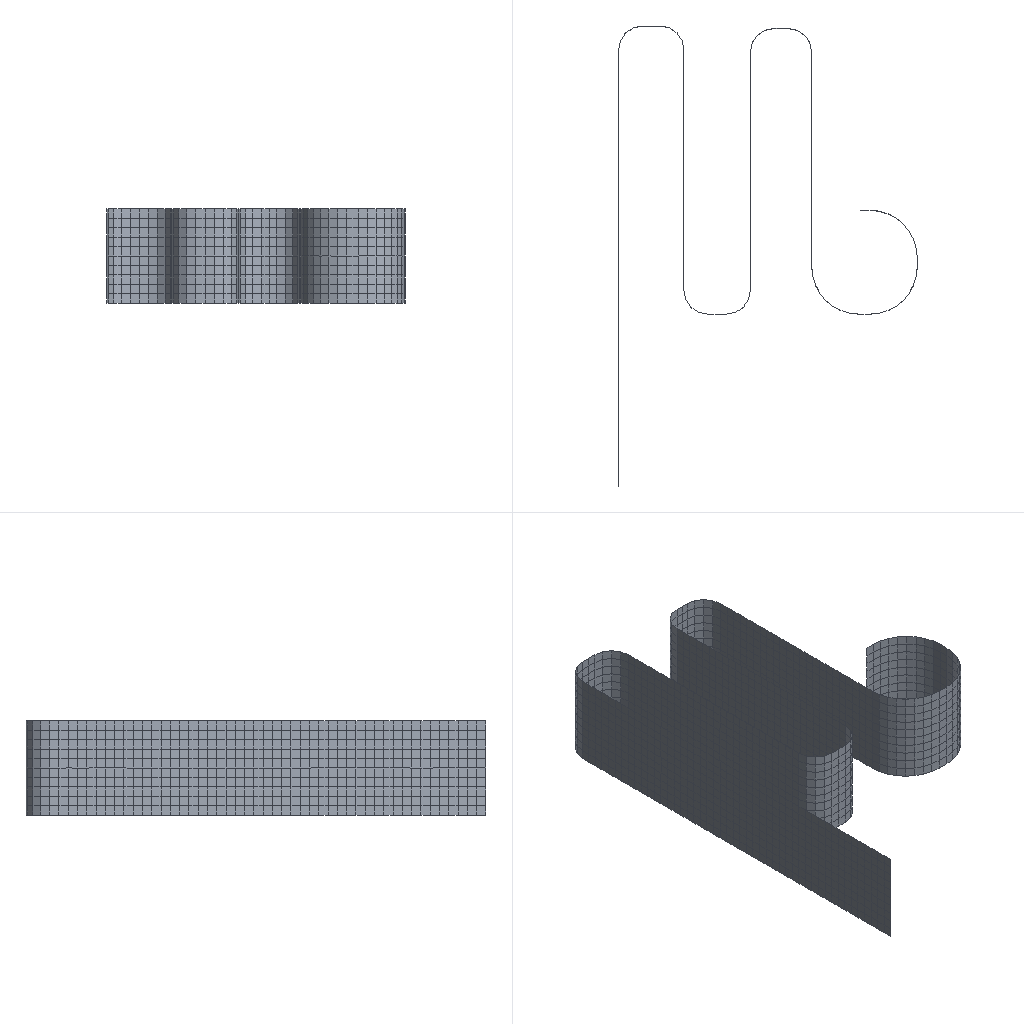Simulation study | ansys workbench
Ansys APDL input file, long lists of numbers shortened:
/batch
/config,noeldb,1     ! force off writing results to database
*get,_wallstrt,active,,time,wall
! ANSYS input file written by Workbench version 2025 R2
! File used for geometry attach:
/title,[REDACTED]
! ****** Begin Custom Load Command Snippet ******
/COM, ACT Extensions:
/COM,     LSDYNA, 2025.2
/COM,/COM,     ANSYSMotion, 2025.2
/COM,
! ****** End   Custom Load Command Snippet ******
*DIM,_wb_ProjectScratch_dir,string,248
_wb_ProjectScratch_dir(1) = ''
*DIM,_wb_SolverFiles_dir,string,248
_wb_SolverFiles_dir(1) = ''
*DIM,_wb_userfiles_dir,string,248
_wb_userfiles_dir(1) = ''
/com,--- Data in consistent NMM units. See Solving Units in the help system for more information.
/units,MPA
/nopr
/wb,file,start              !  signify a WB generated input file
/prep7
! Turn off shape checking because checks already performed inside WB mesher.
! See help system for more information.
SHPP,OFF,,NOWARN
/nolist
etcon,set             ! allow ANSYS to choose best KEYOP's for 180x elements, resets any applicable keyopt to MAPDL defaults
/com,*********** Send User Defined Coordinate System(s) ***********
csys,0
/com,*********** Nodes for the whole assembly ***********
nblock,3,,2178
(1i9,3e20.9e3)
        1     2.046204580E+01     1.679463945E+01     5.000001091E+00
! (1979 more lines like these left out)
-1
/wb,elem,start            !  set before creation of elements
/com,*********** Elements for Body 1 'Surface Body' ***********
et,1,181
keyo,1,1,0          ! bending and membrane stiffness
keyo,1,3,2
MAT,1 $ TYPE,1 $ REAL,1 $ SECNUM,1 $ ESYS,0
eblock,11,COMPACT,,1790
(11i9)
        1        5        7       10       13
! (1789 more lines like these left out)
-1
secnum,1    ! reset the section ID to default
/wb,elem,end               !  done creating elements
toffst,273.15,      ! Temperature offset from absolute zero
/com,*********** Set Reference Temperature ***********
tref,22.
/wb,mat,start              !  starting to send materials
/com,*********** Send Materials ***********
Temperature = 'TEMP' ! Temperature
MP,DENS,1,7.85e-09,	! tonne mm^-3
MP,ALPX,1,1.2e-05,	! C^-1
MP,C,1,434000000,	! mm^2 s^-2 C^-1
MP,KXX,1,60.5,	! tonne mm s^-3 C^-1
MP,RSVX,1,0.00017,	! ohm mm
MP,EX,1,200000,	! tonne s^-2 mm^-1
MP,NUXY,1,0.3,
MP,MURX,1,10000,
/wb,mat,end                !  done sending materials
/com,*********** Send Sheet Properties ***********
sectype,1,shell
secdata,1.
secoff,mid
!************************* Model Summary ********************
!Surface Body,	Structural steel,	matid,	1
!************************* End Model Summary ********************
! get the diagonal of the bounding box. Needed later for other things
*get,_xmin,node,,mnloc,x
*get,_ymin,node,,mnloc,y
*get,_zmin,node,,mnloc,z
*get,_xmax,node,,mxloc,x
*get,_ymax,node,,mxloc,y
*get,_zmax,node,,mxloc,z
_ASMDIAG=(_xmax-_xmin)*(_xmax-_xmin)+(_ymax-_ymin)*(_ymax-_ymin)+(_zmax-_zmin)*(_zmax-_zmin)
_ASMDIAG=SQRT(_ASMDIAG)
/wb,contact,start          !  starting to send contact
/wb,contact,end            !  done creating contacts
/golist
/wb,load,start             !  starting to send loads
/com,*********** Fixed Supports ***********
CMBLOCK,_FIXEDSU,NODE,       11
(8i10)
       113       126       138       149       162       176       188       201
       215      1528      1531
cmsel,s,_FIXEDSU
d,all,all
nsel,all
/com,*********** Define Force Using Surface Effect Elements ***********
local,12,0,0.,0.,0.,0.,0.,0.
csys,0
et,2,156
keyop,2,5,1         !  No orientation node
MAT,2 $ TYPE,2 $ REAL,2 $ SECNUM,2 $ ESYS,12
eblock,11,COMPACT,,10
(11i9)
     1791      195      200
! (9 more lines like these left out)
-1
secnum,1    ! reset the section ID to default
esel,s,type,,2
keyop,2,2,1         ! Apply load in local coordinate system
keyop,2,7,1         ! Use original area so load is constant in large deformation
esel,all
/gst,on,on
fini
*get,_numnode,node,0,count
*get,_numelem,elem,0,count
*get, _MAXELEMNUM, elem, 0, NUM, MAX
*get, _MAXNODENUM, node, 0, NUM, MAX
*get, _MAXELEMTYPE, etyp, 0, NUM, MAX
*get, _MAXREALCONST, rcon, 0, NUM, MAX
/go
/wb,load,end               !  done creating loads
/com,--- Number of total nodes = %_numnode%
/com,--- Number of contact elements = 10
/com,--- Number of spring elements = 0
/com,--- Number of bearing elements = 0
/com,--- Number of solid elements = 1790
/com,--- Number of condensed parts = 0
/com,--- Number of total elements = %_numelem%
*get,_wallbsol,active,,time,wall
/com,****************************************************************************
/com,*************************    SOLUTION       ********************************
/com,****************************************************************************
/solu
antype,0                   ! static analysis
nlgeom,on                  ! Turn on Large Deformation Effects
_thickRatio=  0     ! Ratio of thick parts in the model
eqsl,sparse,,,,,1
cntr,print,1               ! print out contact info and also make no initial contact an error
cncheck,dmp		!	Enable program controlled contact splitting for distributed memory parallel run
dmpoption,emat,no             ! Don't combine emat file for DANSYS
dmpoption,esav,no             ! Don't combine esav file for DANSYS
nldiag,cont,iter           ! print out contact info each equilibrium iteration
rescontrol,define,last,last,,dele	   ! Program Controlled
/com,****************************************************
/com,******************* SOLVE FOR LS 1 OF 1 ****************
esel,s,type,,2
nsle
sfe,all,1,pres,1,25.
sfe,all,2,pres,1,0.
sfe,all,3,pres,1,0.
nsel,all
esel,all
/nopr
/gopr
autots,on                  ! Workbench Program Controlled automatic time stepping
nsub,1,10,1                ! due to presence of general nonlinear
time,1.
outres,erase
outres,all,none
outres,nsol,all,
outres,rsol,all
outres,eangl,all
outres,etmp,all
outres,veng,all
outres,strs,all,
outres,epel,all,
outres,eppl,all,
outres,cont,all,
! *********** WB SOLVE COMMAND ***********
! check interactive state
*get,ANSINTER_,active,,int
*if,ANSINTER_,ne,0,then
/eof
*endif
solve
/com *************** Write FE CONNECTORS *********
CEWRITE,file,ce,,INTE
/com,****************************************************
/com,*************** FINISHED SOLVE FOR LS 1 *************
*get,_wallasol,active,,time,wall
/nopr
*get,_numnode,node,0,count
*get,_numelem,elem,0,count
*get, _MAXELEMNUM, elem, 0, NUM, MAX
*get, _MAXNODENUM, node, 0, NUM, MAX,,,INTERNAL
*get, _MAXELEMTYPE, etyp, 0, NUM, MAX
*get, _MAXREALCONST, rcon, 0, NUM, MAX
*get,_NSOLTHREADS,active,0,ntfs
*get,_NSOLPROCESSES,active,0,npfs
/gopr
/post1
xmlo,ENCODING,ISO-8859-1
xmlo,parm
/xml,parm,xml
fini
/gopr
*get,_walldone,active,,time,wall
_preptime=(_wallbsol-_wallstrt)*3600
_solvtime=(_wallasol-_wallbsol)*3600
_posttime=(_walldone-_wallasol)*3600
_totaltim=(_walldone-_wallstrt)*3600
*get,_dlbratio,active,0,solu,dlbr
*get,_combtime,active,0,solu,comb
*get,_ssmode,active,0,solu,ssmm
*get,_ndofs,active,0,solu,ndof
*get,_sol_end_time,active,0,set,time
*if,_sol_end_time,eq,1.,then
/fclean				!clean distributed files
*endif
/com,--- Total number of nodes = %_numnode%
/com,--- Total number of elements = %_numelem%
/com,--- Element load balance ratio = %_dlbratio%
/com,--- Time to combine distributed files = %_combtime%
/com,--- Sparse memory mode = %_ssmode%
/com,--- Number of DOF = %_ndofs%
/wb,file,end               ! done with WB generated input